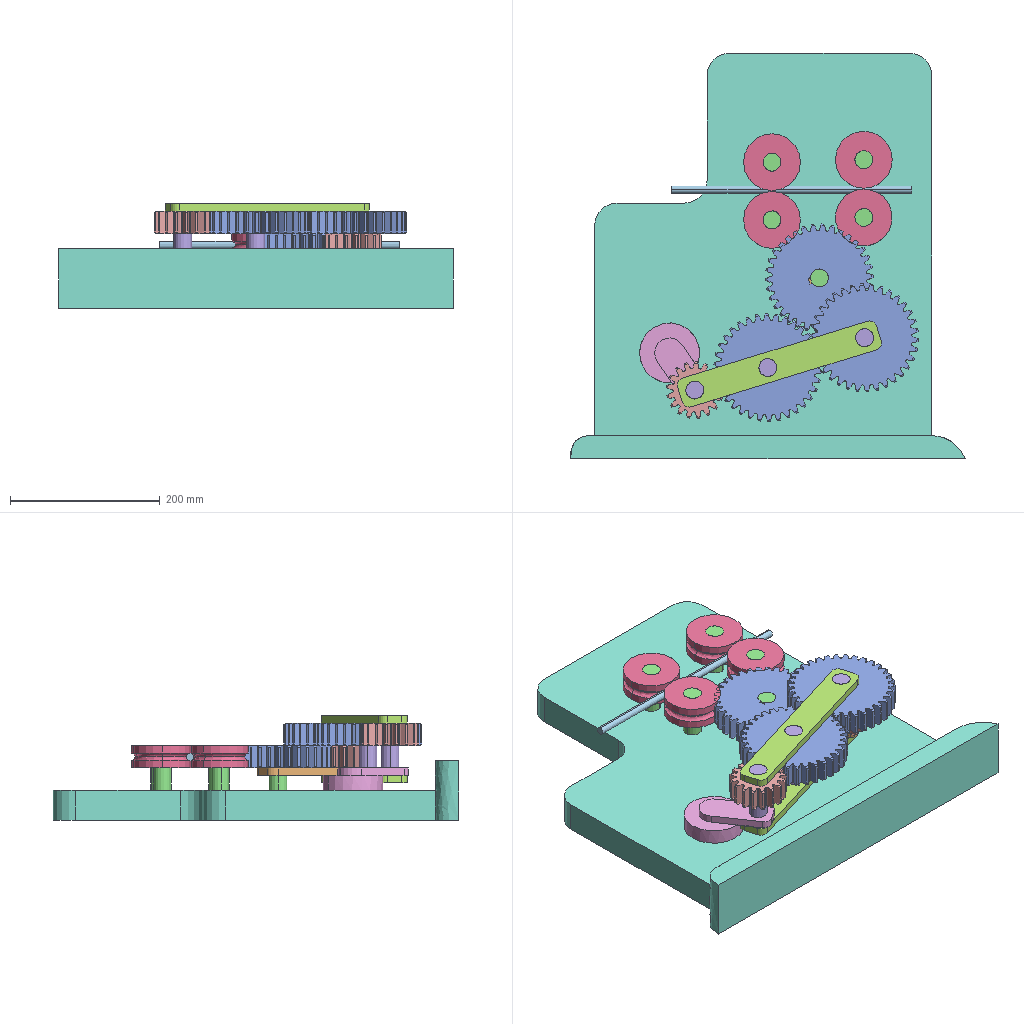Assembly | SolidWorks | 10 different items | 23 placed | box 527 x 541 x 140 mm
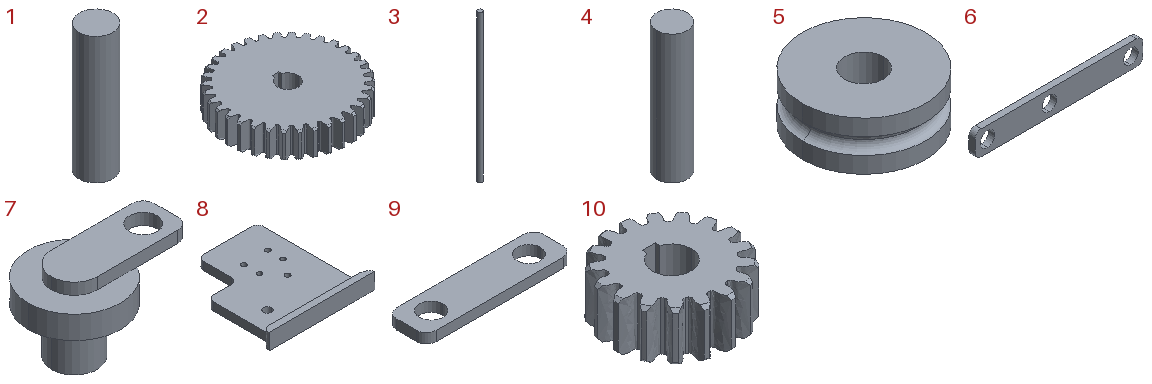Parts list (item | quantity | size | volume | features):
1 | x3 | 24 x 24 x 90 mm | 40715 mm3 | features Extrusion 1
2 | x3 | 144 x 143.631 x 30 mm | 417182 mm3 | features ICE 5, Chamfer 3, CirPattern 1, Extrusion 1, RefAxis 1
3 | x1 | 10 x 10 x 320 mm | 25133 mm3 | features Extrusion 1
4 | x5 | 24 x 24 x 100 mm | 45239 mm3 | features Extrusion 1
5 | x4 | 76 x 76 x 30 mm | 113670 mm3 | features Extrusion 1, RevCut 1
6 | x2 | 277.743 x 10 x 40 mm | 96667 mm3 | features Extrusion 1, Fillet 1, ICE 1
7 | x1 | 120 x 80 x 70 mm | 184127 mm3 | features ICE 4, Extrusion 1, Fillet 1
8 | x1 | 526.791 x 541.265 x 80 mm | 9097852 mm3 | features ICE 8, Extrusion 1, Fillet 1
9 | x1 | 150 x 40 x 10 mm | 50094 mm3 | features Extrusion 1, Fillet 1
10 | x2 | 75.876 x 75.576 x 30 mm | 92447 mm3 | features ICE 5, Chamfer 3, CirPattern 1, Extrusion 1, RefAxis 1
Mates (type | each side: item.copy, entity, surface, feature):
Width | 10.1 face plane Boss-Extrude1 | 10.1 face plane Boss-Extrude1 | 2.1 face plane Boss-Extrude1 | 2.1 face plane Boss-Extrude1
Width | 2.1 face plane Boss-Extrude1 | 2.1 face plane Boss-Extrude1 | 2.2 face plane Boss-Extrude1 | 2.2 face plane Boss-Extrude1
GearDim | 10.1 select_type:24 | 2.1 select_type:24
DistanceDim | 10.1 face cylinder Cut-Extrude3 | 2.1 face cylinder Cut-Extrude3
DistanceDim | 2.1 face cylinder Cut-Extrude3 | 2.2 face cylinder Cut-Extrude3
GearDim | 2.1 select_type:24 | 2.2 select_type:24
Concentric | 2.2 face cylinder Cut-Extrude3 | 6.1 face cylinder Boss-Extrude1
Concentric | 10.1 face cylinder Cut-Extrude3 | 6.1 face cylinder Boss-Extrude1
Concentric | 6.1 face cylinder Boss-Extrude1 | 7.1 face cylinder Cut-Extrude1
Coincident | 6.1 face plane Boss-Extrude1 | 7.1 face plane Boss-Extrude1
Concentric | 7.1 face cylinder Cut-Extrude2 | 8.1 face cylinder Cut-Extrude1
Coincident | 7.1 face plane Boss-Extrude2 | 8.1 face plane Boss-Extrude1
Concentric | 2.2 face cylinder Cut-Extrude3 | 10.2 face cylinder Cut-Extrude3
Parallel | 2.2 face plane Cut-Extrude4 | 10.2 face plane Cut-Extrude4
Coincident | 2.2 face plane Boss-Extrude1 | 10.2 face plane Boss-Extrude1
Coincident | 2.3 face plane Boss-Extrude1 | 10.2 face plane Boss-Extrude1
Concentric | 2.3 face cylinder Cut-Extrude3 | 9.1 face cylinder Boss-Extrude1
Concentric | 2.3 face cylinder Cut-Extrude3 | 8.1 face cylinder Cut-Extrude2
Coincident | 2.3 face plane Boss-Extrude1 | 9.1 face plane Boss-Extrude1
Parallel | 6.1 face cylinder Boss-Extrude1 | 9.1 face cylinder Boss-Extrude1
Coincident | 6.1 face plane Boss-Extrude1 | 9.1 face plane Boss-Extrude1
Parallel | 7.1 face plane Boss-Extrude3 | 8.1 face plane Boss-Extrude1
Concentric | 6.1 face cylinder Boss-Extrude1 | 6.2 face cylinder Boss-Extrude1
Concentric | 2.2 face cylinder Cut-Extrude3 | 6.2 face cylinder Boss-Extrude1
Coincident | 2.1 face plane Boss-Extrude1 | 6.2 face plane Boss-Extrude1
Concentric | 6.2 face cylinder Boss-Extrude1 | 1.1 face cylinder Boss-Extrude1
Coincident | 6.2 face plane Boss-Extrude1 | 1.1 face plane Boss-Extrude1
Concentric | 6.2 face cylinder Boss-Extrude1 | 1.2 face cylinder Boss-Extrude1
Coincident | 6.2 face plane Boss-Extrude1 | 1.2 face plane Boss-Extrude1
Concentric | 2.2 face cylinder Cut-Extrude3 | 1.3 face cylinder Boss-Extrude1
Coincident | 6.2 face plane Boss-Extrude1 | 1.3 face plane Boss-Extrude1
Concentric | 2.3 face cylinder Cut-Extrude3 | assembly face
Coincident | 2.3 face plane Boss-Extrude1 | assembly face | 3 times
Concentric | 8.1 face cylinder Cut-Extrude3 | assembly face | 2 times
Concentric | 2.3 face cylinder Cut-Extrude3 | 4.1 face cylinder Boss-Extrude1
Coincident | 2.3 face plane Boss-Extrude1 | 4.1 face plane Boss-Extrude1
Concentric | assembly face | 4.2 face cylinder Boss-Extrude1
Coincident | assembly face | 4.2 face plane Boss-Extrude1
Concentric | assembly face | 4.3 face cylinder Boss-Extrude1
Coincident | assembly face | 4.3 face plane Boss-Extrude1
GearDim | assembly select_type:0 | 2.3 select_type:24
GearDim | 2.3 select_type:24 | assembly select_type:0
Coincident | assembly face | 5.1 face plane Boss-Extrude1
Concentric | 8.1 face cylinder Cut-Extrude7 | 5.1 face cylinder Boss-Extrude1
Concentric | 8.1 face cylinder Cut-Extrude7 | 5.2 face cylinder Boss-Extrude1
Coincident | assembly face | 5.2 face plane Boss-Extrude1
Concentric | 5.1 face cylinder Boss-Extrude1 | 4.4 face cylinder Boss-Extrude1
Coincident | 5.1 face plane Boss-Extrude1 | 4.4 face plane Boss-Extrude1
Concentric | 5.2 face cylinder Boss-Extrude1 | 4.5 face cylinder Boss-Extrude1
Coincident | 5.2 face plane Boss-Extrude1 | 4.5 face plane Boss-Extrude1
Concentric | 9.1 face cylinder Boss-Extrude1 | 1.3 face cylinder Boss-Extrude1
Concentric | 4.2 face cylinder Boss-Extrude1 | 5.3 face cylinder Boss-Extrude1
Coincident | 4.2 face plane Boss-Extrude1 | 5.3 face plane Boss-Extrude1
Concentric | 8.1 face cylinder Cut-Extrude3 | 4.3 face cylinder Boss-Extrude1
Coincident | 8.1 face plane Boss-Extrude1 | 4.3 face plane Boss-Extrude1
Concentric | 4.3 face cylinder Boss-Extrude1 | 5.4 face cylinder Boss-Extrude1
Coincident | 4.3 face plane Boss-Extrude1 | 5.4 face plane Boss-Extrude1
Concentric | 8.1 face cylinder Cut-Extrude3 | 4.2 face cylinder Boss-Extrude1
RackPinionDim | assembly select_type:0 | 2.3 select_type:24
DistanceDim | assembly face | 8.1 face plane Boss-Extrude1
DistanceDim | 8.1 face plane Boss-Extrude1 | assembly face
GearDim | 2.3 select_type:24 | 10.2 select_type:24
RackPinionDim | 3.1 select_type:24 | 2.3 select_type:24